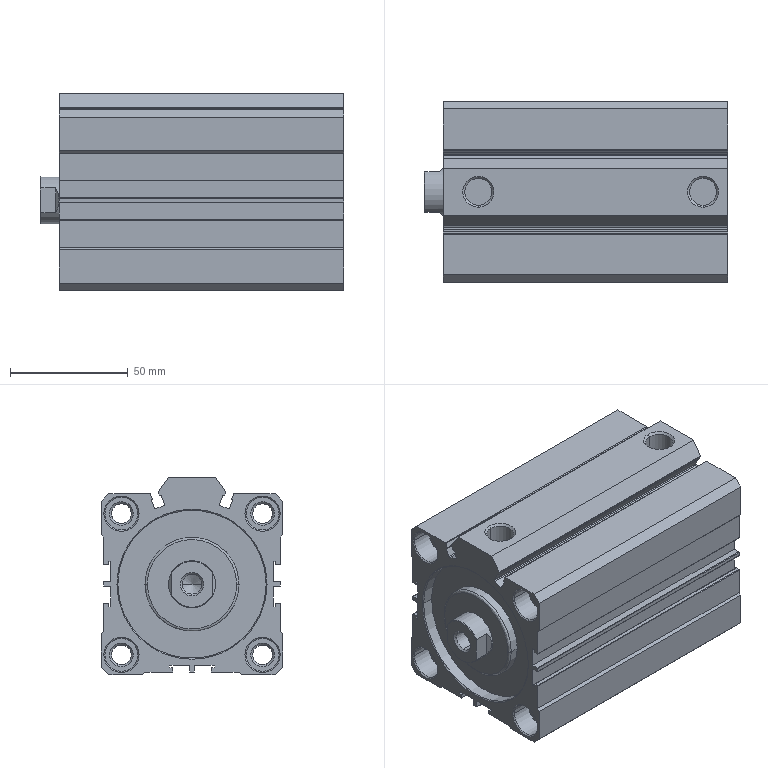Part | SolidWorks | 2 solids | 246 faces | box 129 x 77 x 84 mm | volume 432109 mm3 | cylinder 98 | plane 96 | cone 50 | spline 2 | commonest cylinder face diameters 0.4 x35 14 x16 0.8 x15 8.376 x10 63 x6 11.445 x4